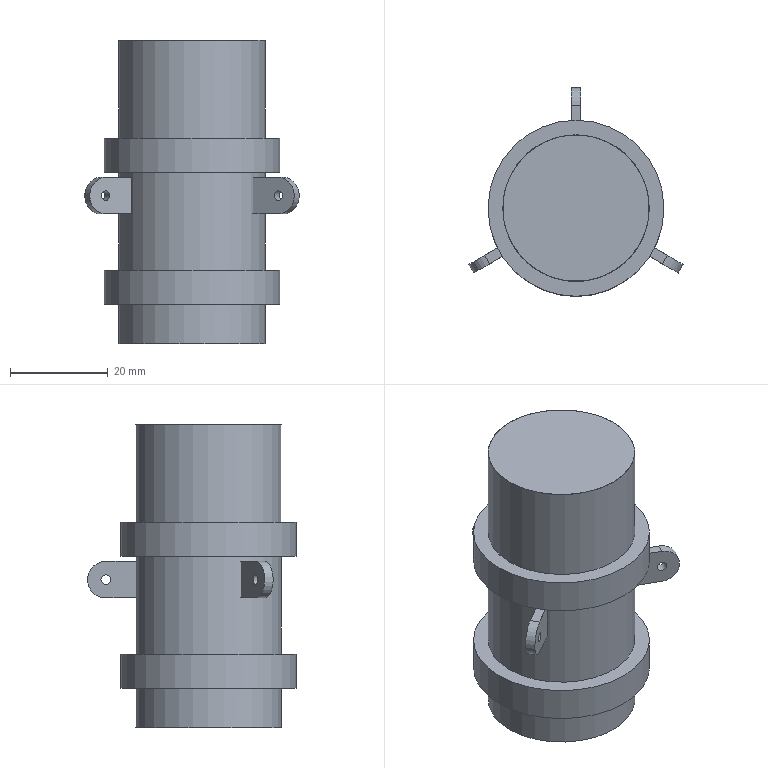Part | NX | features EXTRUDE 9, DATUM_CSYS 8, SKETCH 7, EXTRACT_STRING 6, HOLE PACKAGE 3, SIMPLE HOLE 3, Instance Feature 2, BREP 1, DATUM_PLANE 1, LINKED_FACE 1, Pattern Feature 1, SHELL 1, UNITE 1 | 4 solids | 46 faces | box 43.868 x 42.75 x 62.001 mm | volume 27511 mm3 | plane 29 | cylinder 17 | commonest cylinder face diameters 2 x3 7.5 x3 25 x3 30 x3 31 x2 36 x2